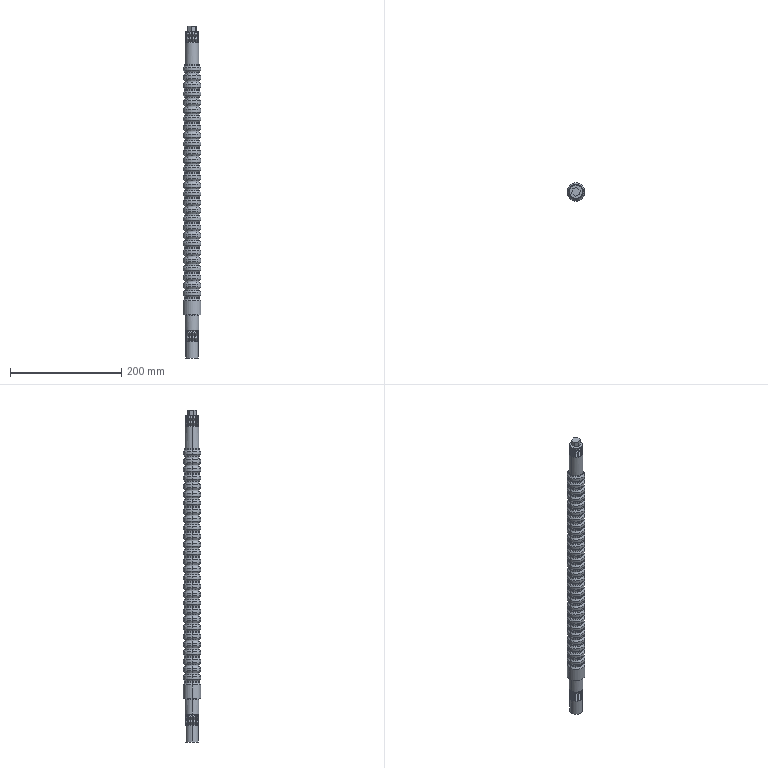Part | STEP file | 400V80 X-Axis Lead Screw | 1 solid | 416 faces | box 32 x 32 x 598 mm | volume 373661 mm3 | cylinder 124 | spline 114 | cone 108 | plane 70 | commonest cylinder face diameters 26 x58 32 x58 25 x4 22 x2 24 x2